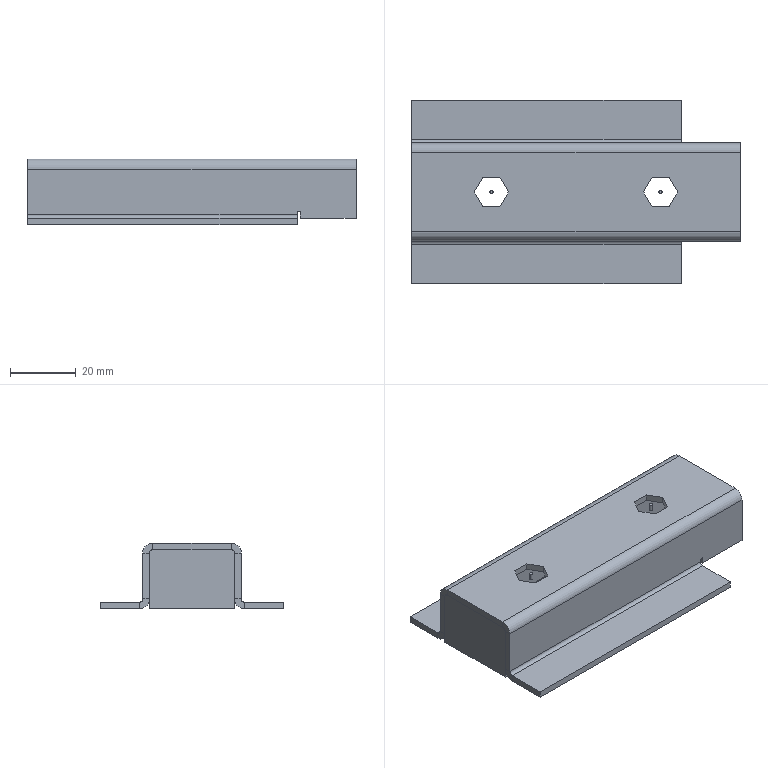Part | SolidWorks | features BaseBody 4 | 4 solids | 74 faces | box 100 x 56 x 20 mm | volume 17344 mm3 | plane 60 | cylinder 14 | commonest cylinder face diameters 2 x6 1 x4 6 x4